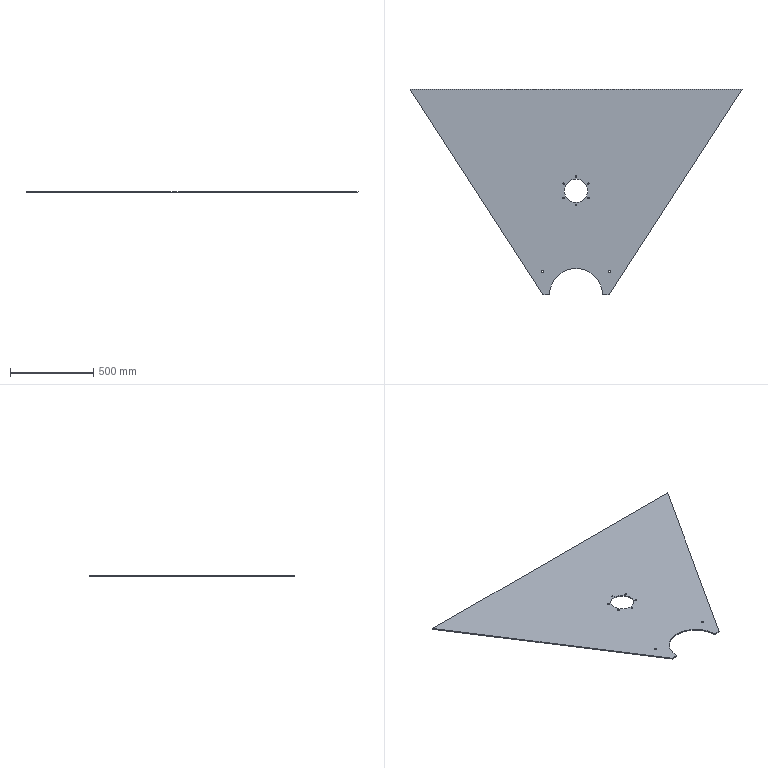Part | SolidWorks | features ICE 4, CirPattern 1, FlatPattern 1, SMBaseFlange 1, SheetMetal 1 | 1 solid | 26 faces | box 2000 x 1240 x 6 mm | volume 8589688 mm3 | cylinder 19 | plane 7 | commonest cylinder face diameters 10 x12 14 x4 140 x2 320 x1
STEP:
#1=CARTESIAN_POINT('',(207.,-480.,-6.));
#2=VERTEX_POINT('',#1);
#3=CARTESIAN_POINT('',(193.,-480.,-6.));
#4=VERTEX_POINT('',#3);
#5=CARTESIAN_POINT('',(200.,-480.,-6.));
#6=DIRECTION('',(0.,0.,-1.));
#7=DIRECTION('',(1.,0.,0.));
#8=AXIS2_PLACEMENT_3D('',#5,#6,#7);
#9=CIRCLE('',#8,7.);
#10=EDGE_CURVE('',#2,#4,#9,.T.);
#11=ORIENTED_EDGE('',*,*,#10,.T.);
#12=CARTESIAN_POINT('',(193.,-480.,0.));
#13=VERTEX_POINT('',#12);
#14=CARTESIAN_POINT('',(193.,-480.,-6.001));
#15=DIRECTION('',(0.,0.,1.));
#16=VECTOR('',#15,1000.);
#17=LINE('',#14,#16);
#18=EDGE_CURVE('',#4,#13,#17,.T.);
#19=ORIENTED_EDGE('',*,*,#18,.T.);
#20=CARTESIAN_POINT('',(207.,-480.,0.));
#21=VERTEX_POINT('',#20);
#22=CARTESIAN_POINT('',(200.,-480.,0.));
#23=DIRECTION('',(0.,0.,1.));
#24=DIRECTION('',(1.,0.,0.));
#25=AXIS2_PLACEMENT_3D('',#22,#23,#24);
#26=CIRCLE('',#25,7.);
#27=EDGE_CURVE('',#13,#21,#26,.T.);
#28=ORIENTED_EDGE('',*,*,#27,.T.);
#29=CARTESIAN_POINT('',(207.,-480.,-6.001));
#30=DIRECTION('',(0.,0.,1.));
#31=VECTOR('',#30,1000.);
#32=LINE('',#29,#31);
#33=EDGE_CURVE('',#2,#21,#32,.T.);
#34=ORIENTED_EDGE('',*,*,#33,.F.);
#35=EDGE_LOOP('',(#11,#19,#28,#34));
#36=FACE_OUTER_BOUND('',#35,.T.);
#37=CARTESIAN_POINT('',(200.,-480.,-6.001));
#38=DIRECTION('',(0.,0.,1.));
#39=DIRECTION('',(1.,0.,0.));
#40=AXIS2_PLACEMENT_3D('',#37,#38,#39);
#41=CYLINDRICAL_SURFACE('',#40,7.);
#42=ADVANCED_FACE('',(#36),#41,.F.);
#43=CARTESIAN_POINT('',(-193.,-480.,-6.));
#44=VERTEX_POINT('',#43);
#45=CARTESIAN_POINT('',(-207.,-480.,-6.));
#46=VERTEX_POINT('',#45);
#47=CARTESIAN_POINT('',(-200.,-480.,-6.));
#48=DIRECTION('',(0.,0.,-1.));
#49=DIRECTION('',(1.,0.,0.));
#50=AXIS2_PLACEMENT_3D('',#47,#48,#49);
#51=CIRCLE('',#50,7.);
#52=EDGE_CURVE('',#44,#46,#51,.T.);
#53=ORIENTED_EDGE('',*,*,#52,.T.);
#54=CARTESIAN_POINT('',(-207.,-480.,0.));
#55=VERTEX_POINT('',#54);
#56=CARTESIAN_POINT('',(-207.,-480.,-6.001));
#57=DIRECTION('',(0.,0.,1.));
#58=VECTOR('',#57,1000.);
#59=LINE('',#56,#58);
#60=EDGE_CURVE('',#46,#55,#59,.T.);
#61=ORIENTED_EDGE('',*,*,#60,.T.);
#62=CARTESIAN_POINT('',(-193.,-480.,0.));
#63=VERTEX_POINT('',#62);
#64=CARTESIAN_POINT('',(-200.,-480.,0.));
#65=DIRECTION('',(0.,0.,1.));
#66=DIRECTION('',(1.,0.,0.));
#67=AXIS2_PLACEMENT_3D('',#64,#65,#66);
#68=CIRCLE('',#67,7.);
#69=EDGE_CURVE('',#55,#63,#68,.T.);
#70=ORIENTED_EDGE('',*,*,#69,.T.);
#71=CARTESIAN_POINT('',(-193.,-480.,-6.001));
#72=DIRECTION('',(0.,0.,1.));
#73=VECTOR('',#72,1000.);
#74=LINE('',#71,#73);
#75=EDGE_CURVE('',#44,#63,#74,.T.);
#76=ORIENTED_EDGE('',*,*,#75,.F.);
#77=EDGE_LOOP('',(#53,#61,#70,#76));
#78=FACE_OUTER_BOUND('',#77,.T.);
#79=CARTESIAN_POINT('',(-200.,-480.,-6.001));
#80=DIRECTION('',(0.,0.,1.));
#81=DIRECTION('',(1.,0.,0.));
#82=AXIS2_PLACEMENT_3D('',#79,#80,#81);
#83=CYLINDRICAL_SURFACE('',#82,7.);
#84=ADVANCED_FACE('',(#78),#83,.F.);
#85=CARTESIAN_POINT('',(78.612,49.5,-6.));
#86=VERTEX_POINT('',#85);
#87=CARTESIAN_POINT('',(68.612,49.5,-6.));
#88=VERTEX_POINT('',#87);
#89=CARTESIAN_POINT('',(73.612,49.5,-6.));
#90=DIRECTION('',(0.,0.,-1.));
#91=DIRECTION('',(1.,0.,0.));
#92=AXIS2_PLACEMENT_3D('',#89,#90,#91);
#93=CIRCLE('',#92,5.);
#94=EDGE_CURVE('',#86,#88,#93,.T.);
#95=ORIENTED_EDGE('',*,*,#94,.T.);
#96=CARTESIAN_POINT('',(68.612,49.5,0.));
#97=VERTEX_POINT('',#96);
#98=CARTESIAN_POINT('',(68.612,49.5,-6.001));
#99=DIRECTION('',(0.,0.,1.));
#100=VECTOR('',#99,1000.);
#101=LINE('',#98,#100);
#102=EDGE_CURVE('',#88,#97,#101,.T.);
#103=ORIENTED_EDGE('',*,*,#102,.T.);
#104=CARTESIAN_POINT('',(78.612,49.5,0.));
#105=VERTEX_POINT('',#104);
#106=CARTESIAN_POINT('',(73.612,49.5,0.));
#107=DIRECTION('',(0.,0.,1.));
#108=DIRECTION('',(0.5,-0.866,0.));
#109=AXIS2_PLACEMENT_3D('',#106,#107,#108);
#110=CIRCLE('',#109,5.);
#111=EDGE_CURVE('',#97,#105,#110,.T.);
#112=ORIENTED_EDGE('',*,*,#111,.T.);
#113=CARTESIAN_POINT('',(78.612,49.5,-6.001));
#114=DIRECTION('',(0.,0.,1.));
#115=VECTOR('',#114,1000.);
#116=LINE('',#113,#115);
#117=EDGE_CURVE('',#86,#105,#116,.T.);
#118=ORIENTED_EDGE('',*,*,#117,.F.);
#119=EDGE_LOOP('',(#95,#103,#112,#118));
#120=FACE_OUTER_BOUND('',#119,.T.);
#121=CARTESIAN_POINT('',(73.612,49.5,-6.001));
#122=DIRECTION('',(0.,0.,1.));
#123=DIRECTION('',(1.,0.,0.));
#124=AXIS2_PLACEMENT_3D('',#121,#122,#123);
#125=CYLINDRICAL_SURFACE('',#124,5.);
#126=ADVANCED_FACE('',(#120),#125,.F.);
#127=CARTESIAN_POINT('',(78.612,-35.5,-6.));
#128=VERTEX_POINT('',#127);
#129=CARTESIAN_POINT('',(68.612,-35.5,-6.));
#130=VERTEX_POINT('',#129);
#131=CARTESIAN_POINT('',(73.612,-35.5,-6.));
#132=DIRECTION('',(0.,0.,-1.));
#133=DIRECTION('',(1.,0.,0.));
#134=AXIS2_PLACEMENT_3D('',#131,#132,#133);
#135=CIRCLE('',#134,5.);
#136=EDGE_CURVE('',#128,#130,#135,.T.);
#137=ORIENTED_EDGE('',*,*,#136,.T.);
#138=CARTESIAN_POINT('',(68.612,-35.5,0.));
#139=VERTEX_POINT('',#138);
#140=CARTESIAN_POINT('',(68.612,-35.5,-6.001));
#141=DIRECTION('',(0.,0.,1.));
#142=VECTOR('',#141,1000.);
#143=LINE('',#140,#142);
#144=EDGE_CURVE('',#130,#139,#143,.T.);
#145=ORIENTED_EDGE('',*,*,#144,.T.);
#146=CARTESIAN_POINT('',(78.612,-35.5,0.));
#147=VERTEX_POINT('',#146);
#148=CARTESIAN_POINT('',(73.612,-35.5,0.));
#149=DIRECTION('',(0.,0.,1.));
#150=DIRECTION('',(-0.5,-0.866,0.));
#151=AXIS2_PLACEMENT_3D('',#148,#149,#150);
#152=CIRCLE('',#151,5.);
#153=EDGE_CURVE('',#139,#147,#152,.T.);
#154=ORIENTED_EDGE('',*,*,#153,.T.);
#155=CARTESIAN_POINT('',(78.612,-35.5,-6.001));
#156=DIRECTION('',(0.,0.,1.));
#157=VECTOR('',#156,1000.);
#158=LINE('',#155,#157);
#159=EDGE_CURVE('',#128,#147,#158,.T.);
#160=ORIENTED_EDGE('',*,*,#159,.F.);
#161=EDGE_LOOP('',(#137,#145,#154,#160));
#162=FACE_OUTER_BOUND('',#161,.T.);
#163=CARTESIAN_POINT('',(73.612,-35.5,-6.001));
#164=DIRECTION('',(0.,0.,1.));
#165=DIRECTION('',(1.,0.,0.));
#166=AXIS2_PLACEMENT_3D('',#163,#164,#165);
#167=CYLINDRICAL_SURFACE('',#166,5.);
#168=ADVANCED_FACE('',(#162),#167,.F.);
#169=CARTESIAN_POINT('',(5.,-78.,-6.));
#170=VERTEX_POINT('',#169);
#171=CARTESIAN_POINT('',(-5.,-78.,-6.));
#172=VERTEX_POINT('',#171);
#173=CARTESIAN_POINT('',(0.,-78.,-6.));
#174=DIRECTION('',(0.,0.,-1.));
#175=DIRECTION('',(1.,0.,0.));
#176=AXIS2_PLACEMENT_3D('',#173,#174,#175);
#177=CIRCLE('',#176,5.);
#178=EDGE_CURVE('',#170,#172,#177,.T.);
#179=ORIENTED_EDGE('',*,*,#178,.T.);
#180=CARTESIAN_POINT('',(-5.,-78.,0.));
#181=VERTEX_POINT('',#180);
#182=CARTESIAN_POINT('',(-5.,-78.,-6.001));
#183=DIRECTION('',(0.,0.,1.));
#184=VECTOR('',#183,1000.);
#185=LINE('',#182,#184);
#186=EDGE_CURVE('',#172,#181,#185,.T.);
#187=ORIENTED_EDGE('',*,*,#186,.T.);
#188=CARTESIAN_POINT('',(5.,-78.,0.));
#189=VERTEX_POINT('',#188);
#190=CARTESIAN_POINT('',(0.,-78.,0.));
#191=DIRECTION('',(0.,0.,1.));
#192=DIRECTION('',(-1.,0.,0.));
#193=AXIS2_PLACEMENT_3D('',#190,#191,#192);
#194=CIRCLE('',#193,5.);
#195=EDGE_CURVE('',#181,#189,#194,.T.);
#196=ORIENTED_EDGE('',*,*,#195,.T.);
#197=CARTESIAN_POINT('',(5.,-78.,-6.001));
#198=DIRECTION('',(0.,0.,1.));
#199=VECTOR('',#198,1000.);
#200=LINE('',#197,#199);
#201=EDGE_CURVE('',#170,#189,#200,.T.);
#202=ORIENTED_EDGE('',*,*,#201,.F.);
#203=EDGE_LOOP('',(#179,#187,#196,#202));
#204=FACE_OUTER_BOUND('',#203,.T.);
#205=CARTESIAN_POINT('',(0.,-78.,-6.001));
#206=DIRECTION('',(0.,0.,1.));
#207=DIRECTION('',(1.,0.,0.));
#208=AXIS2_PLACEMENT_3D('',#205,#206,#207);
#209=CYLINDRICAL_SURFACE('',#208,5.);
#210=ADVANCED_FACE('',(#204),#209,.F.);
#211=CARTESIAN_POINT('',(-68.612,-35.5,-6.));
#212=VERTEX_POINT('',#211);
#213=CARTESIAN_POINT('',(-78.612,-35.5,-6.));
#214=VERTEX_POINT('',#213);
#215=CARTESIAN_POINT('',(-73.612,-35.5,-6.));
#216=DIRECTION('',(0.,0.,-1.));
#217=DIRECTION('',(1.,0.,0.));
#218=AXIS2_PLACEMENT_3D('',#215,#216,#217);
#219=CIRCLE('',#218,5.);
#220=EDGE_CURVE('',#212,#214,#219,.T.);
#221=ORIENTED_EDGE('',*,*,#220,.T.);
#222=CARTESIAN_POINT('',(-78.612,-35.5,0.));
#223=VERTEX_POINT('',#222);
#224=CARTESIAN_POINT('',(-78.612,-35.5,-6.001));
#225=DIRECTION('',(0.,0.,1.));
#226=VECTOR('',#225,1000.);
#227=LINE('',#224,#226);
#228=EDGE_CURVE('',#214,#223,#227,.T.);
#229=ORIENTED_EDGE('',*,*,#228,.T.);
#230=CARTESIAN_POINT('',(-68.612,-35.5,0.));
#231=VERTEX_POINT('',#230);
#232=CARTESIAN_POINT('',(-73.612,-35.5,0.));
#233=DIRECTION('',(0.,0.,1.));
#234=DIRECTION('',(-0.5,0.866,0.));
#235=AXIS2_PLACEMENT_3D('',#232,#233,#234);
#236=CIRCLE('',#235,5.);
#237=EDGE_CURVE('',#223,#231,#236,.T.);
#238=ORIENTED_EDGE('',*,*,#237,.T.);
#239=CARTESIAN_POINT('',(-68.612,-35.5,-6.001));
#240=DIRECTION('',(0.,0.,1.));
#241=VECTOR('',#240,1000.);
#242=LINE('',#239,#241);
#243=EDGE_CURVE('',#212,#231,#242,.T.);
#244=ORIENTED_EDGE('',*,*,#243,.F.);
#245=EDGE_LOOP('',(#221,#229,#238,#244));
#246=FACE_OUTER_BOUND('',#245,.T.);
#247=CARTESIAN_POINT('',(-73.612,-35.5,-6.001));
#248=DIRECTION('',(0.,0.,1.));
#249=DIRECTION('',(1.,0.,0.));
#250=AXIS2_PLACEMENT_3D('',#247,#248,#249);
#251=CYLINDRICAL_SURFACE('',#250,5.);
#252=ADVANCED_FACE('',(#246),#251,.F.);
#253=CARTESIAN_POINT('',(-68.612,49.5,-6.));
#254=VERTEX_POINT('',#253);
#255=CARTESIAN_POINT('',(-78.612,49.5,-6.));
#256=VERTEX_POINT('',#255);
#257=CARTESIAN_POINT('',(-73.612,49.5,-6.));
#258=DIRECTION('',(0.,0.,-1.));
#259=DIRECTION('',(1.,0.,0.));
#260=AXIS2_PLACEMENT_3D('',#257,#258,#259);
#261=CIRCLE('',#260,5.);
#262=EDGE_CURVE('',#254,#256,#261,.T.);
#263=ORIENTED_EDGE('',*,*,#262,.T.);
#264=CARTESIAN_POINT('',(-78.612,49.5,0.));
#265=VERTEX_POINT('',#264);
#266=CARTESIAN_POINT('',(-78.612,49.5,-6.001));
#267=DIRECTION('',(0.,0.,1.));
#268=VECTOR('',#267,1000.);
#269=LINE('',#266,#268);
#270=EDGE_CURVE('',#256,#265,#269,.T.);
#271=ORIENTED_EDGE('',*,*,#270,.T.);
#272=CARTESIAN_POINT('',(-68.612,49.5,0.));
#273=VERTEX_POINT('',#272);
#274=CARTESIAN_POINT('',(-73.612,49.5,0.));
#275=DIRECTION('',(0.,0.,1.));
#276=DIRECTION('',(0.5,0.866,0.));
#277=AXIS2_PLACEMENT_3D('',#274,#275,#276);
#278=CIRCLE('',#277,5.);
#279=EDGE_CURVE('',#265,#273,#278,.T.);
#280=ORIENTED_EDGE('',*,*,#279,.T.);
#281=CARTESIAN_POINT('',(-68.612,49.5,-6.001));
#282=DIRECTION('',(0.,0.,1.));
#283=VECTOR('',#282,1000.);
#284=LINE('',#281,#283);
#285=EDGE_CURVE('',#254,#273,#284,.T.);
#286=ORIENTED_EDGE('',*,*,#285,.F.);
#287=EDGE_LOOP('',(#263,#271,#280,#286));
#288=FACE_OUTER_BOUND('',#287,.T.);
#289=CARTESIAN_POINT('',(-73.612,49.5,-6.001));
#290=DIRECTION('',(0.,0.,1.));
#291=DIRECTION('',(1.,0.,0.));
#292=AXIS2_PLACEMENT_3D('',#289,#290,#291);
#293=CYLINDRICAL_SURFACE('',#292,5.);
#294=ADVANCED_FACE('',(#288),#293,.F.);
#295=CARTESIAN_POINT('',(5.,92.,-6.));
#296=VERTEX_POINT('',#295);
#297=CARTESIAN_POINT('',(-5.,92.,-6.));
#298=VERTEX_POINT('',#297);
#299=CARTESIAN_POINT('',(0.,92.,-6.));
#300=DIRECTION('',(0.,0.,-1.));
#301=DIRECTION('',(1.,0.,0.));
#302=AXIS2_PLACEMENT_3D('',#299,#300,#301);
#303=CIRCLE('',#302,5.);
#304=EDGE_CURVE('',#296,#298,#303,.T.);
#305=ORIENTED_EDGE('',*,*,#304,.T.);
#306=CARTESIAN_POINT('',(-5.,92.,0.));
#307=VERTEX_POINT('',#306);
#308=CARTESIAN_POINT('',(-5.,92.,-6.001));
#309=DIRECTION('',(0.,0.,1.));
#310=VECTOR('',#309,1000.);
#311=LINE('',#308,#310);
#312=EDGE_CURVE('',#298,#307,#311,.T.);
#313=ORIENTED_EDGE('',*,*,#312,.T.);
#314=CARTESIAN_POINT('',(5.,92.,0.));
#315=VERTEX_POINT('',#314);
#316=CARTESIAN_POINT('',(0.,92.,0.));
#317=DIRECTION('',(0.,0.,1.));
#318=DIRECTION('',(1.,0.,0.));
#319=AXIS2_PLACEMENT_3D('',#316,#317,#318);
#320=CIRCLE('',#319,5.);
#321=EDGE_CURVE('',#307,#315,#320,.T.);
#322=ORIENTED_EDGE('',*,*,#321,.T.);
#323=CARTESIAN_POINT('',(5.,92.,-6.001));
#324=DIRECTION('',(0.,0.,1.));
#325=VECTOR('',#324,1000.);
#326=LINE('',#323,#325);
#327=EDGE_CURVE('',#296,#315,#326,.T.);
#328=ORIENTED_EDGE('',*,*,#327,.F.);
#329=EDGE_LOOP('',(#305,#313,#322,#328));
#330=FACE_OUTER_BOUND('',#329,.T.);
#331=CARTESIAN_POINT('',(0.,92.,-6.001));
#332=DIRECTION('',(0.,0.,1.));
#333=DIRECTION('',(1.,0.,0.));
#334=AXIS2_PLACEMENT_3D('',#331,#332,#333);
#335=CYLINDRICAL_SURFACE('',#334,5.);
#336=ADVANCED_FACE('',(#330),#335,.F.);
#337=CARTESIAN_POINT('',(70.,7.,-6.));
#338=VERTEX_POINT('',#337);
#339=CARTESIAN_POINT('',(-70.,7.,-6.));
#340=VERTEX_POINT('',#339);
#341=CARTESIAN_POINT('',(0.,7.,-6.));
#342=DIRECTION('',(0.,0.,-1.));
#343=DIRECTION('',(1.,0.,0.));
#344=AXIS2_PLACEMENT_3D('',#341,#342,#343);
#345=CIRCLE('',#344,70.);
#346=EDGE_CURVE('',#338,#340,#345,.T.);
#347=ORIENTED_EDGE('',*,*,#346,.T.);
#348=CARTESIAN_POINT('',(-70.,7.,0.));
#349=VERTEX_POINT('',#348);
#350=CARTESIAN_POINT('',(-70.,7.,-6.001));
#351=DIRECTION('',(0.,0.,1.));
#352=VECTOR('',#351,1000.);
#353=LINE('',#350,#352);
#354=EDGE_CURVE('',#340,#349,#353,.T.);
#355=ORIENTED_EDGE('',*,*,#354,.T.);
#356=CARTESIAN_POINT('',(70.,7.,0.));
#357=VERTEX_POINT('',#356);
#358=CARTESIAN_POINT('',(0.,7.,0.));
#359=DIRECTION('',(0.,0.,1.));
#360=DIRECTION('',(1.,0.,0.));
#361=AXIS2_PLACEMENT_3D('',#358,#359,#360);
#362=CIRCLE('',#361,70.);
#363=EDGE_CURVE('',#349,#357,#362,.T.);
#364=ORIENTED_EDGE('',*,*,#363,.T.);
#365=CARTESIAN_POINT('',(70.,7.,-6.001));
#366=DIRECTION('',(0.,0.,1.));
#367=VECTOR('',#366,1000.);
#368=LINE('',#365,#367);
#369=EDGE_CURVE('',#338,#357,#368,.T.);
#370=ORIENTED_EDGE('',*,*,#369,.F.);
#371=EDGE_LOOP('',(#347,#355,#364,#370));
#372=FACE_OUTER_BOUND('',#371,.T.);
#373=CARTESIAN_POINT('',(0.,7.,-6.001));
#374=DIRECTION('',(0.,0.,1.));
#375=DIRECTION('',(1.,0.,0.));
#376=AXIS2_PLACEMENT_3D('',#373,#374,#375);
#377=CYLINDRICAL_SURFACE('',#376,70.);
#378=ADVANCED_FACE('',(#372),#377,.F.);
#379=CARTESIAN_POINT('',(-160.,-620.,0.));
#380=VERTEX_POINT('',#379);
#381=CARTESIAN_POINT('',(-160.,-620.,-6.));
#382=VERTEX_POINT('',#381);
#383=CARTESIAN_POINT('',(-160.,-620.,4.));
#384=DIRECTION('',(0.,0.,-1.));
#385=VECTOR('',#384,1000.);
#386=LINE('',#383,#385);
#387=EDGE_CURVE('',#380,#382,#386,.T.);
#388=ORIENTED_EDGE('',*,*,#387,.F.);
#389=CARTESIAN_POINT('',(-200.,-620.,0.));
#390=VERTEX_POINT('',#389);
#391=CARTESIAN_POINT('',(1000.,-620.,0.));
#392=DIRECTION('',(1.,0.,0.));
#393=VECTOR('',#392,1000.);
#394=LINE('',#391,#393);
#395=EDGE_CURVE('',#390,#380,#394,.T.);
#396=ORIENTED_EDGE('',*,*,#395,.F.);
#397=CARTESIAN_POINT('',(-200.,-620.,-6.));
#398=VERTEX_POINT('',#397);
#399=CARTESIAN_POINT('',(-200.,-620.,-6.));
#400=DIRECTION('',(0.,0.,1.));
#401=VECTOR('',#400,1000.);
#402=LINE('',#399,#401);
#403=EDGE_CURVE('',#398,#390,#402,.T.);
#404=ORIENTED_EDGE('',*,*,#403,.F.);
#405=CARTESIAN_POINT('',(1000.,-620.,-6.));
#406=DIRECTION('',(1.,0.,0.));
#407=VECTOR('',#406,1000.);
#408=LINE('',#405,#407);
#409=EDGE_CURVE('',#398,#382,#408,.T.);
#410=ORIENTED_EDGE('',*,*,#409,.T.);
#411=EDGE_LOOP('',(#388,#396,#404,#410));
#412=FACE_OUTER_BOUND('',#411,.T.);
#413=CARTESIAN_POINT('',(1000.,-620.,-6.));
#414=DIRECTION('',(0.,-1.,0.));
#415=DIRECTION('',(1.,0.,0.));
#416=AXIS2_PLACEMENT_3D('',#413,#414,#415);
#417=PLANE('',#416);
#418=ADVANCED_FACE('',(#412),#417,.T.);
#419=CARTESIAN_POINT('',(160.,-620.,-6.));
#420=VERTEX_POINT('',#419);
#421=CARTESIAN_POINT('',(160.,-620.,0.));
#422=VERTEX_POINT('',#421);
#423=CARTESIAN_POINT('',(160.,-620.,4.));
#424=DIRECTION('',(0.,0.,1.));
#425=VECTOR('',#424,1000.);
#426=LINE('',#423,#425);
#427=EDGE_CURVE('',#420,#422,#426,.T.);
#428=ORIENTED_EDGE('',*,*,#427,.F.);
#429=CARTESIAN_POINT('',(200.,-620.,-6.));
#430=VERTEX_POINT('',#429);
#431=CARTESIAN_POINT('',(1000.,-620.,-6.));
#432=DIRECTION('',(1.,0.,0.));
#433=VECTOR('',#432,1000.);
#434=LINE('',#431,#433);
#435=EDGE_CURVE('',#420,#430,#434,.T.);
#436=ORIENTED_EDGE('',*,*,#435,.T.);
#437=CARTESIAN_POINT('',(200.,-620.,0.));
#438=VERTEX_POINT('',#437);
#439=CARTESIAN_POINT('',(200.,-620.,-6.));
#440=DIRECTION('',(0.,0.,1.));
#441=VECTOR('',#440,1000.);
#442=LINE('',#439,#441);
#443=EDGE_CURVE('',#430,#438,#442,.T.);
#444=ORIENTED_EDGE('',*,*,#443,.T.);
#445=CARTESIAN_POINT('',(1000.,-620.,0.));
#446=DIRECTION('',(1.,0.,0.));
#447=VECTOR('',#446,1000.);
#448=LINE('',#445,#447);
#449=EDGE_CURVE('',#422,#438,#448,.T.);
#450=ORIENTED_EDGE('',*,*,#449,.F.);
#451=EDGE_LOOP('',(#428,#436,#444,#450));
#452=FACE_OUTER_BOUND('',#451,.T.);
#453=CARTESIAN_POINT('',(1000.,-620.,-6.));
#454=DIRECTION('',(0.,-1.,0.));
#455=DIRECTION('',(1.,0.,0.));
#456=AXIS2_PLACEMENT_3D('',#453,#454,#455);
#457=PLANE('',#456);
#458=ADVANCED_FACE('',(#452),#457,.T.);
#459=ORIENTED_EDGE('',*,*,#10,.F.);
#460=CARTESIAN_POINT('',(200.,-480.,-6.));
#461=DIRECTION('',(0.,0.,-1.));
#462=DIRECTION('',(1.,0.,0.));
#463=AXIS2_PLACEMENT_3D('',#460,#461,#462);
#464=CIRCLE('',#463,7.);
#465=EDGE_CURVE('',#4,#2,#464,.T.);
#466=ORIENTED_EDGE('',*,*,#465,.F.);
#467=EDGE_LOOP('',(#459,#466));
#468=FACE_BOUND('',#467,.T.);
#469=ORIENTED_EDGE('',*,*,#52,.F.);
#470=CARTESIAN_POINT('',(-200.,-480.,-6.));
#471=DIRECTION('',(0.,0.,-1.));
#472=DIRECTION('',(1.,0.,0.));
#473=AXIS2_PLACEMENT_3D('',#470,#471,#472);
#474=CIRCLE('',#473,7.);
#475=EDGE_CURVE('',#46,#44,#474,.T.);
#476=ORIENTED_EDGE('',*,*,#475,.F.);
#477=EDGE_LOOP('',(#469,#476));
#478=FACE_BOUND('',#477,.T.);
#479=ORIENTED_EDGE('',*,*,#94,.F.);
#480=CARTESIAN_POINT('',(73.612,49.5,-6.));
#481=DIRECTION('',(0.,0.,-1.));
#482=DIRECTION('',(1.,0.,0.));
#483=AXIS2_PLACEMENT_3D('',#480,#481,#482);
#484=CIRCLE('',#483,5.);
#485=EDGE_CURVE('',#88,#86,#484,.T.);
#486=ORIENTED_EDGE('',*,*,#485,.F.);
#487=EDGE_LOOP('',(#479,#486));
#488=FACE_BOUND('',#487,.T.);
#489=ORIENTED_EDGE('',*,*,#136,.F.);
#490=CARTESIAN_POINT('',(73.612,-35.5,-6.));
#491=DIRECTION('',(0.,0.,-1.));
#492=DIRECTION('',(1.,0.,0.));
#493=AXIS2_PLACEMENT_3D('',#490,#491,#492);
#494=CIRCLE('',#493,5.);
#495=EDGE_CURVE('',#130,#128,#494,.T.);
#496=ORIENTED_EDGE('',*,*,#495,.F.);
#497=EDGE_LOOP('',(#489,#496));
#498=FACE_BOUND('',#497,.T.);
#499=ORIENTED_EDGE('',*,*,#178,.F.);
#500=CARTESIAN_POINT('',(0.,-78.,-6.));
#501=DIRECTION('',(0.,0.,-1.));
#502=DIRECTION('',(1.,0.,0.));
#503=AXIS2_PLACEMENT_3D('',#500,#501,#502);
#504=CIRCLE('',#503,5.);
#505=EDGE_CURVE('',#172,#170,#504,.T.);
#506=ORIENTED_EDGE('',*,*,#505,.F.);
#507=EDGE_LOOP('',(#499,#506));
#508=FACE_BOUND('',#507,.T.);
#509=ORIENTED_EDGE('',*,*,#220,.F.);
#510=CARTESIAN_POINT('',(-73.612,-35.5,-6.));
#511=DIRECTION('',(0.,0.,-1.));
#512=DIRECTION('',(1.,0.,0.));
#513=AXIS2_PLACEMENT_3D('',#510,#511,#512);
#514=CIRCLE('',#513,5.);
#515=EDGE_CURVE('',#214,#212,#514,.T.);
#516=ORIENTED_EDGE('',*,*,#515,.F.);
#517=EDGE_LOOP('',(#509,#516));
#518=FACE_BOUND('',#517,.T.);
#519=ORIENTED_EDGE('',*,*,#262,.F.);
#520=CARTESIAN_POINT('',(-73.612,49.5,-6.));
#521=DIRECTION('',(0.,0.,-1.));
#522=DIRECTION('',(1.,0.,0.));
#523=AXIS2_PLACEMENT_3D('',#520,#521,#522);
#524=CIRCLE('',#523,5.);
#525=EDGE_CURVE('',#256,#254,#524,.T.);
#526=ORIENTED_EDGE('',*,*,#525,.F.);
#527=EDGE_LOOP('',(#519,#526));
#528=FACE_BOUND('',#527,.T.);
#529=ORIENTED_EDGE('',*,*,#304,.F.);
#530=CARTESIAN_POINT('',(0.,92.,-6.));
#531=DIRECTION('',(0.,0.,-1.));
#532=DIRECTION('',(1.,0.,0.));
#533=AXIS2_PLACEMENT_3D('',#530,#531,#532);
#534=CIRCLE('',#533,5.);
#535=EDGE_CURVE('',#298,#296,#534,.T.);
#536=ORIENTED_EDGE('',*,*,#535,.F.);
#537=EDGE_LOOP('',(#529,#536));
#538=FACE_BOUND('',#537,.T.);
#539=ORIENTED_EDGE('',*,*,#346,.F.);
#540=CARTESIAN_POINT('',(0.,7.,-6.));
#541=DIRECTION('',(0.,0.,-1.));
#542=DIRECTION('',(1.,0.,0.));
#543=AXIS2_PLACEMENT_3D('',#540,#541,#542);
#544=CIRCLE('',#543,70.);
#545=EDGE_CURVE('',#340,#338,#544,.T.);
#546=ORIENTED_EDGE('',*,*,#545,.F.);
#547=EDGE_LOOP('',(#539,#546));
#548=FACE_BOUND('',#547,.T.);
#549=ORIENTED_EDGE('',*,*,#435,.F.);
#550=CARTESIAN_POINT('',(0.,-620.,-6.));
#551=DIRECTION('',(0.,0.,-1.));
#552=DIRECTION('',(-1.,0.,0.));
#553=AXIS2_PLACEMENT_3D('',#550,#551,#552);
#554=CIRCLE('',#553,160.);
#555=EDGE_CURVE('',#382,#420,#554,.T.);
#556=ORIENTED_EDGE('',*,*,#555,.F.);
#557=ORIENTED_EDGE('',*,*,#409,.F.);
#558=CARTESIAN_POINT('',(-1000.,620.,-6.));
#559=VERTEX_POINT('',#558);
#560=CARTESIAN_POINT('',(-1000.,620.,-6.));
#561=DIRECTION('',(0.5421,-0.8403,0.));
#562=VECTOR('',#561,1000.);
#563=LINE('',#560,#562);
#564=EDGE_CURVE('',#559,#398,#563,.T.);
#565=ORIENTED_EDGE('',*,*,#564,.F.);
#566=CARTESIAN_POINT('',(1000.,620.,-6.));
#567=VERTEX_POINT('',#566);
#568=CARTESIAN_POINT('',(1000.,620.,-6.));
#569=DIRECTION('',(-1.,0.,0.));
#570=VECTOR('',#569,1000.);
#571=LINE('',#568,#570);
#572=EDGE_CURVE('',#567,#559,#571,.T.);
#573=ORIENTED_EDGE('',*,*,#572,.F.);
#574=CARTESIAN_POINT('',(1000.,620.,-6.));
#575=DIRECTION('',(0.5421,0.8403,0.));
#576=VECTOR('',#575,1000.);
#577=LINE('',#574,#576);
#578=EDGE_CURVE('',#430,#567,#577,.T.);
#579=ORIENTED_EDGE('',*,*,#578,.F.);
#580=EDGE_LOOP('',(#549,#556,#557,#565,#573,#579));
#581=FACE_OUTER_BOUND('',#580,.T.);
#582=CARTESIAN_POINT('',(0.,0.,-6.));
#583=DIRECTION('',(0.,0.,1.));
#584=DIRECTION('',(1.,0.,0.));
#585=AXIS2_PLACEMENT_3D('',#582,#583,#584);
#586=PLANE('',#585);
#587=ADVANCED_FACE('',(#468,#478,#488,#498,#508,#518,#528,#538,#548,#581),#586,.F.);
#588=CARTESIAN_POINT('',(200.,-480.,0.));
#589=DIRECTION('',(0.,0.,1.));
#590=DIRECTION('',(1.,0.,0.));
#591=AXIS2_PLACEMENT_3D('',#588,#589,#590);
#592=CIRCLE('',#591,7.);
#593=EDGE_CURVE('',#21,#13,#592,.T.);
#594=ORIENTED_EDGE('',*,*,#593,.F.);
#595=ORIENTED_EDGE('',*,*,#27,.F.);
#596=EDGE_LOOP('',(#594,#595));
#597=FACE_BOUND('',#596,.T.);
#598=CARTESIAN_POINT('',(-200.,-480.,0.));
#599=DIRECTION('',(0.,0.,1.));
#600=DIRECTION('',(1.,0.,0.));
#601=AXIS2_PLACEMENT_3D('',#598,#599,#600);
#602=CIRCLE('',#601,7.);
#603=EDGE_CURVE('',#63,#55,#602,.T.);
#604=ORIENTED_EDGE('',*,*,#603,.F.);
#605=ORIENTED_EDGE('',*,*,#69,.F.);
#606=EDGE_LOOP('',(#604,#605));
#607=FACE_BOUND('',#606,.T.);
#608=CARTESIAN_POINT('',(73.612,49.5,0.));
#609=DIRECTION('',(0.,0.,1.));
#610=DIRECTION('',(0.5,-0.866,0.));
#611=AXIS2_PLACEMENT_3D('',#608,#609,#610);
#612=CIRCLE('',#611,5.);
#613=EDGE_CURVE('',#105,#97,#612,.T.);
#614=ORIENTED_EDGE('',*,*,#613,.F.);
#615=ORIENTED_EDGE('',*,*,#111,.F.);
#616=EDGE_LOOP('',(#614,#615));
#617=FACE_BOUND('',#616,.T.);
#618=CARTESIAN_POINT('',(73.612,-35.5,0.));
#619=DIRECTION('',(0.,0.,1.));
#620=DIRECTION('',(-0.5,-0.866,0.));
#621=AXIS2_PLACEMENT_3D('',#618,#619,#620);
#622=CIRCLE('',#621,5.);
#623=EDGE_CURVE('',#147,#139,#622,.T.);
#624=ORIENTED_EDGE('',*,*,#623,.F.);
#625=ORIENTED_EDGE('',*,*,#153,.F.);
#626=EDGE_LOOP('',(#624,#625));
#627=FACE_BOUND('',#626,.T.);
#628=CARTESIAN_POINT('',(0.,-78.,0.));
#629=DIRECTION('',(0.,0.,1.));
#630=DIRECTION('',(-1.,0.,0.));
#631=AXIS2_PLACEMENT_3D('',#628,#629,#630);
#632=CIRCLE('',#631,5.);
#633=EDGE_CURVE('',#189,#181,#632,.T.);
#634=ORIENTED_EDGE('',*,*,#633,.F.);
#635=ORIENTED_EDGE('',*,*,#195,.F.);
#636=EDGE_LOOP('',(#634,#635));
#637=FACE_BOUND('',#636,.T.);
#638=CARTESIAN_POINT('',(-73.612,-35.5,0.));
#639=DIRECTION('',(0.,0.,1.));
#640=DIRECTION('',(-0.5,0.866,0.));
#641=AXIS2_PLACEMENT_3D('',#638,#639,#640);
#642=CIRCLE('',#641,5.);
#643=EDGE_CURVE('',#231,#223,#642,.T.);
#644=ORIENTED_EDGE('',*,*,#643,.F.);
#645=ORIENTED_EDGE('',*,*,#237,.F.);
#646=EDGE_LOOP('',(#644,#645));
#647=FACE_BOUND('',#646,.T.);
#648=CARTESIAN_POINT('',(-73.612,49.5,0.));
#649=DIRECTION('',(0.,0.,1.));
#650=DIRECTION('',(0.5,0.866,0.));
#651=AXIS2_PLACEMENT_3D('',#648,#649,#650);
#652=CIRCLE('',#651,5.);
#653=EDGE_CURVE('',#273,#265,#652,.T.);
#654=ORIENTED_EDGE('',*,*,#653,.F.);
#655=ORIENTED_EDGE('',*,*,#279,.F.);
#656=EDGE_LOOP('',(#654,#655));
#657=FACE_BOUND('',#656,.T.);
#658=CARTESIAN_POINT('',(0.,-620.,0.));
#659=DIRECTION('',(0.,0.,1.));
#660=DIRECTION('',(1.,0.,0.));
#661=AXIS2_PLACEMENT_3D('',#658,#659,#660);
#662=CIRCLE('',#661,160.);
#663=EDGE_CURVE('',#422,#380,#662,.T.);
#664=ORIENTED_EDGE('',*,*,#663,.F.);
#665=ORIENTED_EDGE('',*,*,#449,.T.);
#666=CARTESIAN_POINT('',(1000.,620.,0.));
#667=VERTEX_POINT('',#666);
#668=CARTESIAN_POINT('',(1000.,620.,0.));
#669=DIRECTION('',(0.5421,0.8403,0.));
#670=VECTOR('',#669,1000.);
#671=LINE('',#668,#670);
#672=EDGE_CURVE('',#438,#667,#671,.T.);
#673=ORIENTED_EDGE('',*,*,#672,.T.);
#674=CARTESIAN_POINT('',(-1000.,620.,0.));
#675=VERTEX_POINT('',#674);
#676=CARTESIAN_POINT('',(1000.,620.,0.));
#677=DIRECTION('',(-1.,0.,0.));
#678=VECTOR('',#677,1000.);
#679=LINE('',#676,#678);
#680=EDGE_CURVE('',#667,#675,#679,.T.);
#681=ORIENTED_EDGE('',*,*,#680,.T.);
#682=CARTESIAN_POINT('',(-1000.,620.,0.));
#683=DIRECTION('',(0.5421,-0.8403,0.));
#684=VECTOR('',#683,1000.);
#685=LINE('',#682,#684);
#686=EDGE_CURVE('',#675,#390,#685,.T.);
#687=ORIENTED_EDGE('',*,*,#686,.T.);
#688=ORIENTED_EDGE('',*,*,#395,.T.);
#689=EDGE_LOOP('',(#664,#665,#673,#681,#687,#688));
#690=FACE_OUTER_BOUND('',#689,.T.);
#691=CARTESIAN_POINT('',(0.,92.,0.));
#692=DIRECTION('',(0.,0.,1.));
#693=DIRECTION('',(1.,0.,0.));
#694=AXIS2_PLACEMENT_3D('',#691,#692,#693);
#695=CIRCLE('',#694,5.);
#696=EDGE_CURVE('',#315,#307,#695,.T.);
#697=ORIENTED_EDGE('',*,*,#696,.F.);
#698=ORIENTED_EDGE('',*,*,#321,.F.);
#699=EDGE_LOOP('',(#697,#698));
#700=FACE_BOUND('',#699,.T.);
#701=CARTESIAN_POINT('',(0.,7.,0.));
#702=DIRECTION('',(0.,0.,1.));
#703=DIRECTION('',(1.,0.,0.));
#704=AXIS2_PLACEMENT_3D('',#701,#702,#703);
#705=CIRCLE('',#704,70.);
#706=EDGE_CURVE('',#357,#349,#705,.T.);
#707=ORIENTED_EDGE('',*,*,#706,.F.);
#708=ORIENTED_EDGE('',*,*,#363,.F.);
#709=EDGE_LOOP('',(#707,#708));
#710=FACE_BOUND('',#709,.T.);
#711=CARTESIAN_POINT('',(0.,0.,0.));
#712=DIRECTION('',(0.,0.,1.));
#713=DIRECTION('',(1.,0.,0.));
#714=AXIS2_PLACEMENT_3D('',#711,#712,#713);
#715=PLANE('',#714);
#716=ADVANCED_FACE('',(#597,#607,#617,#627,#637,#647,#657,#690,#700,#710),#715,.T.);
#717=ORIENTED_EDGE('',*,*,#680,.F.);
#718=CARTESIAN_POINT('',(1000.,620.,-6.));
#719=DIRECTION('',(0.,0.,1.));
#720=VECTOR('',#719,1000.);
#721=LINE('',#718,#720);
#722=EDGE_CURVE('',#567,#667,#721,.T.);
#723=ORIENTED_EDGE('',*,*,#722,.F.);
#724=ORIENTED_EDGE('',*,*,#572,.T.);
#725=CARTESIAN_POINT('',(-1000.,620.,-6.));
#726=DIRECTION('',(0.,0.,1.));
#727=VECTOR('',#726,1000.);
#728=LINE('',#725,#727);
#729=EDGE_CURVE('',#559,#675,#728,.T.);
#730=ORIENTED_EDGE('',*,*,#729,.T.);
#731=EDGE_LOOP('',(#717,#723,#724,#730));
#732=FACE_OUTER_BOUND('',#731,.T.);
#733=CARTESIAN_POINT('',(1000.,620.,-6.));
#734=DIRECTION('',(0.,1.,0.));
#735=DIRECTION('',(-1.,0.,0.));
#736=AXIS2_PLACEMENT_3D('',#733,#734,#735);
#737=PLANE('',#736);
#738=ADVANCED_FACE('',(#732),#737,.T.);
#739=ORIENTED_EDGE('',*,*,#443,.F.);
#740=ORIENTED_EDGE('',*,*,#578,.T.);
#741=ORIENTED_EDGE('',*,*,#722,.T.);
#742=ORIENTED_EDGE('',*,*,#672,.F.);
#743=EDGE_LOOP('',(#739,#740,#741,#742));
#744=FACE_OUTER_BOUND('',#743,.T.);
#745=CARTESIAN_POINT('',(1000.,620.,-6.));
#746=DIRECTION('',(0.8403,-0.5421,0.));
#747=DIRECTION('',(0.5421,0.8403,0.));
#748=AXIS2_PLACEMENT_3D('',#745,#746,#747);
#749=PLANE('',#748);
#750=ADVANCED_FACE('',(#744),#749,.T.);
#751=ORIENTED_EDGE('',*,*,#729,.F.);
#752=ORIENTED_EDGE('',*,*,#564,.T.);
#753=ORIENTED_EDGE('',*,*,#403,.T.);
#754=ORIENTED_EDGE('',*,*,#686,.F.);
#755=EDGE_LOOP('',(#751,#752,#753,#754));
#756=FACE_OUTER_BOUND('',#755,.T.);
#757=CARTESIAN_POINT('',(-1000.,620.,-6.));
#758=DIRECTION('',(-0.8403,-0.5421,0.));
#759=DIRECTION('',(0.5421,-0.8403,0.));
#760=AXIS2_PLACEMENT_3D('',#757,#758,#759);
#761=PLANE('',#760);
#762=ADVANCED_FACE('',(#756),#761,.T.);
#763=ORIENTED_EDGE('',*,*,#354,.F.);
#764=ORIENTED_EDGE('',*,*,#545,.T.);
#765=ORIENTED_EDGE('',*,*,#369,.T.);
#766=ORIENTED_EDGE('',*,*,#706,.T.);
#767=EDGE_LOOP('',(#763,#764,#765,#766));
#768=FACE_OUTER_BOUND('',#767,.T.);
#769=CARTESIAN_POINT('',(0.,7.,-6.001));
#770=DIRECTION('',(0.,0.,1.));
#771=DIRECTION('',(1.,0.,0.));
#772=AXIS2_PLACEMENT_3D('',#769,#770,#771);
#773=CYLINDRICAL_SURFACE('',#772,70.);
#774=ADVANCED_FACE('',(#768),#773,.F.);
#775=ORIENTED_EDGE('',*,*,#312,.F.);
#776=ORIENTED_EDGE('',*,*,#535,.T.);
#777=ORIENTED_EDGE('',*,*,#327,.T.);
#778=ORIENTED_EDGE('',*,*,#696,.T.);
#779=EDGE_LOOP('',(#775,#776,#777,#778));
#780=FACE_OUTER_BOUND('',#779,.T.);
#781=CARTESIAN_POINT('',(0.,92.,-6.001));
#782=DIRECTION('',(0.,0.,1.));
#783=DIRECTION('',(1.,0.,0.));
#784=AXIS2_PLACEMENT_3D('',#781,#782,#783);
#785=CYLINDRICAL_SURFACE('',#784,5.);
#786=ADVANCED_FACE('',(#780),#785,.F.);
#787=ORIENTED_EDGE('',*,*,#387,.T.);
#788=ORIENTED_EDGE('',*,*,#555,.T.);
#789=ORIENTED_EDGE('',*,*,#427,.T.);
#790=ORIENTED_EDGE('',*,*,#663,.T.);
#791=EDGE_LOOP('',(#787,#788,#789,#790));
#792=FACE_OUTER_BOUND('',#791,.T.);
#793=CARTESIAN_POINT('',(0.,-620.,4.));
#794=DIRECTION('',(0.,0.,-1.));
#795=DIRECTION('',(-1.,0.,0.));
#796=AXIS2_PLACEMENT_3D('',#793,#794,#795);
#797=CYLINDRICAL_SURFACE('',#796,160.);
#798=ADVANCED_FACE('',(#792),#797,.F.);
#799=ORIENTED_EDGE('',*,*,#270,.F.);
#800=ORIENTED_EDGE('',*,*,#525,.T.);
#801=ORIENTED_EDGE('',*,*,#285,.T.);
#802=ORIENTED_EDGE('',*,*,#653,.T.);
#803=EDGE_LOOP('',(#799,#800,#801,#802));
#804=FACE_OUTER_BOUND('',#803,.T.);
#805=CARTESIAN_POINT('',(-73.612,49.5,-6.001));
#806=DIRECTION('',(0.,0.,1.));
#807=DIRECTION('',(1.,0.,0.));
#808=AXIS2_PLACEMENT_3D('',#805,#806,#807);
#809=CYLINDRICAL_SURFACE('',#808,5.);
#810=ADVANCED_FACE('',(#804),#809,.F.);
#811=ORIENTED_EDGE('',*,*,#228,.F.);
#812=ORIENTED_EDGE('',*,*,#515,.T.);
#813=ORIENTED_EDGE('',*,*,#243,.T.);
#814=ORIENTED_EDGE('',*,*,#643,.T.);
#815=EDGE_LOOP('',(#811,#812,#813,#814));
#816=FACE_OUTER_BOUND('',#815,.T.);
#817=CARTESIAN_POINT('',(-73.612,-35.5,-6.001));
#818=DIRECTION('',(0.,0.,1.));
#819=DIRECTION('',(1.,0.,0.));
#820=AXIS2_PLACEMENT_3D('',#817,#818,#819);
#821=CYLINDRICAL_SURFACE('',#820,5.);
#822=ADVANCED_FACE('',(#816),#821,.F.);
#823=ORIENTED_EDGE('',*,*,#186,.F.);
#824=ORIENTED_EDGE('',*,*,#505,.T.);
#825=ORIENTED_EDGE('',*,*,#201,.T.);
#826=ORIENTED_EDGE('',*,*,#633,.T.);
#827=EDGE_LOOP('',(#823,#824,#825,#826));
#828=FACE_OUTER_BOUND('',#827,.T.);
#829=CARTESIAN_POINT('',(0.,-78.,-6.001));
#830=DIRECTION('',(0.,0.,1.));
#831=DIRECTION('',(1.,0.,0.));
#832=AXIS2_PLACEMENT_3D('',#829,#830,#831);
#833=CYLINDRICAL_SURFACE('',#832,5.);
#834=ADVANCED_FACE('',(#828),#833,.F.);
#835=ORIENTED_EDGE('',*,*,#144,.F.);
#836=ORIENTED_EDGE('',*,*,#495,.T.);
#837=ORIENTED_EDGE('',*,*,#159,.T.);
#838=ORIENTED_EDGE('',*,*,#623,.T.);
#839=EDGE_LOOP('',(#835,#836,#837,#838));
#840=FACE_OUTER_BOUND('',#839,.T.);
#841=CARTESIAN_POINT('',(73.612,-35.5,-6.001));
#842=DIRECTION('',(0.,0.,1.));
#843=DIRECTION('',(1.,0.,0.));
#844=AXIS2_PLACEMENT_3D('',#841,#842,#843);
#845=CYLINDRICAL_SURFACE('',#844,5.);
#846=ADVANCED_FACE('',(#840),#845,.F.);
#847=ORIENTED_EDGE('',*,*,#102,.F.);
#848=ORIENTED_EDGE('',*,*,#485,.T.);
#849=ORIENTED_EDGE('',*,*,#117,.T.);
#850=ORIENTED_EDGE('',*,*,#613,.T.);
#851=EDGE_LOOP('',(#847,#848,#849,#850));
#852=FACE_OUTER_BOUND('',#851,.T.);
#853=CARTESIAN_POINT('',(73.612,49.5,-6.001));
#854=DIRECTION('',(0.,0.,1.));
#855=DIRECTION('',(1.,0.,0.));
#856=AXIS2_PLACEMENT_3D('',#853,#854,#855);
#857=CYLINDRICAL_SURFACE('',#856,5.);
#858=ADVANCED_FACE('',(#852),#857,.F.);
#859=ORIENTED_EDGE('',*,*,#60,.F.);
#860=ORIENTED_EDGE('',*,*,#475,.T.);
#861=ORIENTED_EDGE('',*,*,#75,.T.);
#862=ORIENTED_EDGE('',*,*,#603,.T.);
#863=EDGE_LOOP('',(#859,#860,#861,#862));
#864=FACE_OUTER_BOUND('',#863,.T.);
#865=CARTESIAN_POINT('',(-200.,-480.,-6.001));
#866=DIRECTION('',(0.,0.,1.));
#867=DIRECTION('',(1.,0.,0.));
#868=AXIS2_PLACEMENT_3D('',#865,#866,#867);
#869=CYLINDRICAL_SURFACE('',#868,7.);
#870=ADVANCED_FACE('',(#864),#869,.F.);
#871=ORIENTED_EDGE('',*,*,#18,.F.);
#872=ORIENTED_EDGE('',*,*,#465,.T.);
#873=ORIENTED_EDGE('',*,*,#33,.T.);
#874=ORIENTED_EDGE('',*,*,#593,.T.);
#875=EDGE_LOOP('',(#871,#872,#873,#874));
#876=FACE_OUTER_BOUND('',#875,.T.);
#877=CARTESIAN_POINT('',(200.,-480.,-6.001));
#878=DIRECTION('',(0.,0.,1.));
#879=DIRECTION('',(1.,0.,0.));
#880=AXIS2_PLACEMENT_3D('',#877,#878,#879);
#881=CYLINDRICAL_SURFACE('',#880,7.);
#882=ADVANCED_FACE('',(#876),#881,.F.);
#883=CLOSED_SHELL('',(#42,#84,#126,#168,#210,#252,#294,#336,#378,#418,#458,#587,#716,#738,#750,#762,#774,#786,#798,#810,#822,#834,#846,#858,#870,#882));
#884=MANIFOLD_SOLID_BREP('',#883);
#885=CARTESIAN_POINT('',(0.,0.,0.));
#886=DIRECTION('',(0.,0.,1.));
#887=DIRECTION('',(1.,0.,0.));
#888=AXIS2_PLACEMENT_3D('',#885,#886,#887);
#889=(LENGTH_UNIT()NAMED_UNIT(*)SI_UNIT(.MILLI.,.METRE.));
#890=UNCERTAINTY_MEASURE_WITH_UNIT(LENGTH_MEASURE(0.00001),#889,'','');
#891=(NAMED_UNIT(*)PLANE_ANGLE_UNIT()SI_UNIT($,.RADIAN.));
#892=(NAMED_UNIT(*)SI_UNIT($,.STERADIAN.)SOLID_ANGLE_UNIT());
#893=(GEOMETRIC_REPRESENTATION_CONTEXT(3)GLOBAL_UNCERTAINTY_ASSIGNED_CONTEXT((#890))GLOBAL_UNIT_ASSIGNED_CONTEXT((#889,#891,#892))REPRESENTATION_CONTEXT('',''));
#894=ADVANCED_BREP_SHAPE_REPRESENTATION('',(#884,#888),#893);